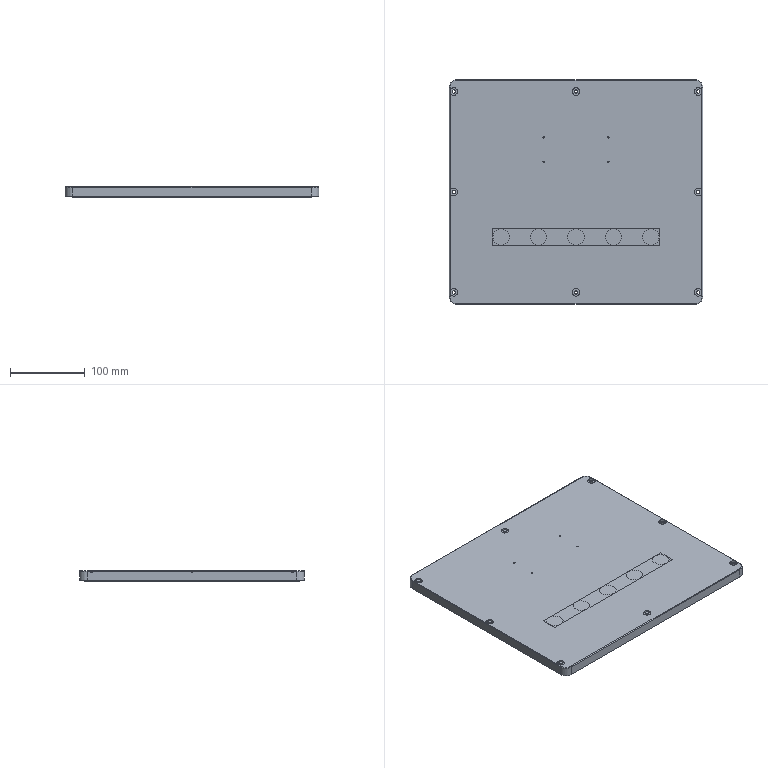NC program | NX | posted with a generic post | part box 338 x 300 x 14.5 mm
Lines 2037 to 2954 of 2954:
(ZLEVEL_PROFILE , TOOL : D10JING)
N4042 T14 M6
N4044 G54
N4046 G17 G0 G90 X160.684 Y-156.916 S9500 M3
N4048 G43 Z30. H14
N4050 Z-11.5
N4052 G94 G1 Z-14.5 F1000.
N4054 X159.866 Y-155.5
N4056 G3 X159. Y-155. R1.
N4058 G1 X-159.
N4060 G2 X-174. Y-140. R15.
N4062 G1 Y140.
N4064 G2 X-159. Y155. R15.
N4066 G1 X159.
N4068 G2 X174. Y140. R15.
N4070 G1 Y-140.
N4072 G2 X159. Y-155. R15.
N4074 G3 X158.134 Y-155.5 R1.
N4076 G1 X157.268 Y-157.
N4078 Z-11.5
N4080 G0 Z30.
(ZLEVEL_PROFILE_COPY , TOOL : D10JING)
N4082 X-52.063 Y-63.427
N4084 Z-2.
N4086 G1 Z-5.
N4088 X-50.866 Y-65.5
N4090 G3 X-50. Y-66. R1.
N4092 X-44. Y-60. R6.
N4094 X-50. Y-66. R-6.
N4096 X-49.134 Y-65.5 R1.
N4098 G1 X-47.937 Y-63.427
N4100 Z-2.
N4102 G0 Z53.
N4104 X-103.427 Y-57.937
N4106 Z-2.
N4108 G1 Z-5.
N4110 X-105.5 Y-59.134
N4112 G3 X-106. Y-60. R1.
N4114 X-100. Y-66. R6.
N4116 X-106. Y-60. R-6.
N4118 X-105.5 Y-60.866 R1.
N4120 G1 X-103.427 Y-62.063
N4122 Z-2.
N4124 G0 Z53.
N4126 X47.937 Y-63.427
N4128 Z-2.
N4130 G1 Z-5.
N4132 X49.134 Y-65.5
N4134 G3 X50. Y-66. R1.
N4136 X56. Y-60. R6.
N4138 X50. Y-66. R-6.
N4140 X50.866 Y-65.5 R1.
N4142 G1 X52.063 Y-63.427
N4144 Z-2.
N4146 G0 Z53.
N4148 X-2.063
N4150 Z-2.
N4152 G1 Z-5.
N4154 X-0.866 Y-65.5
N4156 G3 X0. Y-66. R1.
N4158 X6. Y-60. R6.
N4160 X0. Y-66. R-6.
N4162 X0.866 Y-65.5 R1.
N4164 G1 X2.063 Y-63.427
N4166 Z-2.
N4168 G0 Z53.
N4170 X103.427 Y-62.063
N4172 Z-2.
N4174 G1 Z-5.
N4176 X105.5 Y-60.866
N4178 G3 X106. Y-60. R1.
N4180 X100. Y-54. R6.
N4182 X106. Y-60. R-6.
N4184 X105.5 Y-59.134 R1.
N4186 G1 X103.427 Y-57.937
N4188 Z-2.
N4190 G0 Z30.
N4192 M5
(ZLEVEL_PROFILE_1 , TOOL : D3R0.5)
N4194 T07 M6
N4196 G54
N4198 G17 G0 G90 X-0.52 Y150.79 S9500 M3
N4200 G43 Z30. H7
N4202 Z0.988
N4204 G94 G1 Z-0.012 F1000.
N4206 X-0.26 Y150.34
N4208 G3 X0. Y150.19 R0.3
N4210 G1 X159. F2500.
N4212 G2 X169.19 Y140. R10.19
N4214 G1 Y-140.
N4216 G2 X159. Y-150.19 R10.19
N4218 G1 X-159.
N4220 G2 X-169.19 Y-140. R10.19
N4222 G1 Y140.
N4224 G2 X-159. Y150.19 R10.19
N4226 G1 X0.
N4228 Y150.251 Z-0.021
N4230 Y150.3 Z-0.03
N4232 X-159.
N4234 G3 X-169.3 Y140. R10.3
N4236 G1 Y-140.
N4238 G3 X-159. Y-150.3 R10.3
N4240 G1 X159.
N4242 G3 X169.3 Y-140. R10.3
N4244 G1 Y140.
N4246 G3 X159. Y150.3 R10.3
N4248 G1 X0.
N4250 Y150.356 Z-0.043
N4252 Y150.403 Z-0.055
N4254 X159.
N4256 G2 X169.403 Y140. R10.403
N4258 G1 Y-140.
N4260 G2 X159. Y-150.403 R10.403
N4262 G1 X-159.
N4264 G2 X-169.403 Y-140. R10.403
N4266 G1 Y140.
N4268 G2 X-159. Y150.403 R10.403
N4270 G1 X0.
N4272 Y150.455 Z-0.071
N4274 Y150.502 Z-0.086
N4276 X-159.
N4278 G3 X-169.502 Y140. R10.502
N4280 G1 Y-140.
N4282 G3 X-159. Y-150.502 R10.502
N4284 G1 X159.
N4286 G3 X169.502 Y-140. R10.502
N4288 G1 Y140.
N4290 G3 X159. Y150.502 R10.502
N4292 G1 X0.
N4294 Y150.552 Z-0.105
N4296 Y150.597 Z-0.124
N4298 X159.
N4300 G2 X169.597 Y140. R10.597
N4302 G1 Y-140.
N4304 G2 X159. Y-150.597 R10.597
N4306 G1 X-159.
N4308 G2 X-169.597 Y-140. R10.597
N4310 G1 Y140.
N4312 G2 X-159. Y150.597 R10.597
N4314 G1 X0.
N4316 Y150.645 Z-0.146
N4318 Y150.689 Z-0.167
N4320 X-159.
N4322 G3 X-169.689 Y140. R10.689
N4324 G1 Y-140.
N4326 G3 X-159. Y-150.689 R10.689
N4328 G1 X159.
N4330 G3 X169.689 Y-140. R10.689
N4332 G1 Y140.
N4334 G3 X159. Y150.689 R10.689
N4336 G1 X0.
N4338 Y150.734 Z-0.192
N4340 Y150.777 Z-0.217
N4342 X159.
N4344 G2 X169.777 Y140. R10.777
N4346 G1 Y-140.
N4348 G2 X159. Y-150.777 R10.777
N4350 G1 X-159.
N4352 G2 X-169.777 Y-140. R10.777
N4354 G1 Y140.
N4356 G2 X-159. Y150.777 R10.777
N4358 G1 X0.
N4360 Y150.821 Z-0.244
N4362 Y150.861 Z-0.272
N4364 X-159.
N4366 G3 X-169.861 Y140. R10.861
N4368 G1 Y-140.
N4370 G3 X-159. Y-150.861 R10.861
N4372 G1 X159.
N4374 G3 X169.861 Y-140. R10.861
N4376 G1 Y140.
N4378 G3 X159. Y150.861 R10.861
N4380 G1 X0.
N4382 Y150.903 Z-0.302
N4384 Y150.942 Z-0.333
N4386 X159.
N4388 G2 X169.942 Y140. R10.942
N4390 G1 Y-140.
N4392 G2 X159. Y-150.942 R10.942
N4394 G1 X-159.
N4396 G2 X-169.942 Y-140. R10.942
N4398 G1 Y140.
N4400 G2 X-159. Y150.942 R10.942
N4402 G1 X0.
N4404 Y150.981 Z-0.365
N4406 Y151.018 Z-0.398
N4408 X-159.
N4410 G3 X-170.018 Y140. R11.018
N4412 G1 Y-140.
N4414 G3 X-159. Y-151.018 R11.018
N4416 G1 X159.
N4418 G3 X170.018 Y-140. R11.018
N4420 G1 Y140.
N4422 G3 X159. Y151.018 R11.018
N4424 G1 X0.
N4426 Y151.055 Z-0.434
N4428 Y151.089 Z-0.469
N4430 X159.
N4432 G2 X170.089 Y140. R11.089
N4434 G1 Y-140.
N4436 G2 X159. Y-151.089 R11.089
N4438 G1 X-159.
N4440 G2 X-170.089 Y-140. R11.089
N4442 G1 Y140.
N4444 G2 X-159. Y151.089 R11.089
N4446 G1 X0.
N4448 Y151.124 Z-0.506
N4450 Y151.156 Z-0.544
N4452 X-159.
N4454 G3 X-170.156 Y140. R11.156
N4456 G1 Y-140.
N4458 G3 X-159. Y-151.156 R11.156
N4460 G1 X159.
N4462 G3 X170.156 Y-140. R11.156
N4464 G1 Y140.
N4466 G3 X159. Y151.156 R11.156
N4468 G1 X0.
N4470 Y151.188 Z-0.584
N4472 Y151.217 Z-0.623
N4474 X159.
N4476 G2 X170.217 Y140. R11.217
N4478 G1 Y-140.
N4480 G2 X159. Y-151.217 R11.217
N4482 G1 X-159.
N4484 G2 X-170.217 Y-140. R11.217
N4486 G1 Y140.
N4488 G2 X-159. Y151.217 R11.217
N4490 G1 X0.
N4492 Y151.246 Z-0.665
N4494 Y151.273 Z-0.707
N4496 X-159.
N4498 G3 X-170.273 Y140. R11.273
N4500 G1 Y-140.
N4502 G3 X-159. Y-151.273 R11.273
N4504 G1 X159.
N4506 G3 X170.273 Y-140. R11.273
N4508 G1 Y140.
N4510 G3 X159. Y151.273 R11.273
N4512 G1 X0.
N4514 Y151.299 Z-0.75
N4516 Y151.323 Z-0.793
N4518 X159.
N4520 G2 X170.323 Y140. R11.323
N4522 G1 Y-140.
N4524 G2 X159. Y-151.323 R11.323
N4526 G1 X-159.
N4528 G2 X-170.323 Y-140. R11.323
N4530 G1 Y140.
N4532 G2 X-159. Y151.323 R11.323
N4534 G1 X0.
N4536 Y151.346 Z-0.838
N4538 Y151.367 Z-0.883
N4540 X-159.
N4542 G3 X-170.367 Y140. R11.367
N4544 G1 Y-140.
N4546 G3 X-159. Y-151.367 R11.367
N4548 G1 X159.
N4550 G3 X170.367 Y-140. R11.367
N4552 G1 Y140.
N4554 G3 X159. Y151.367 R11.367
N4556 G1 X0.
N4558 Y151.387 Z-0.93
N4560 Y151.405 Z-0.976
N4562 X159.
N4564 G2 X170.405 Y140. R11.405
N4566 G1 Y-140.
N4568 G2 X159. Y-151.405 R11.405
N4570 G1 X-159.
N4572 G2 X-170.405 Y-140. R11.405
N4574 G1 Y140.
N4576 G2 X-159. Y151.405 R11.405
N4578 G1 X0.
N4580 Y151.422 Z-1.023
N4582 Y151.437 Z-1.071
N4584 X-159.
N4586 G3 X-170.437 Y140. R11.437
N4588 G1 Y-140.
N4590 G3 X-159. Y-151.437 R11.437
N4592 G1 X159.
N4594 G3 X170.437 Y-140. R11.437
N4596 G1 Y140.
N4598 G3 X159. Y151.437 R11.437
N4600 G1 X0.
N4602 Y151.451 Z-1.119
N4604 Y151.463 Z-1.168
N4606 X159.
N4608 G2 X170.463 Y140. R11.463
N4610 G1 Y-140.
N4612 G2 X159. Y-151.463 R11.463
N4614 G1 X-159.
N4616 G2 X-170.463 Y-140. R11.463
N4618 G1 Y140.
N4620 G2 X-159. Y151.463 R11.463
N4622 G1 X0.
N4624 Y151.472 Z-1.209
N4626 Y151.479 Z-1.251
N4628 X-159.
N4630 G3 X-170.479 Y140. R11.479
N4632 G1 Y-140.
N4634 G3 X-159. Y-151.479 R11.479
N4636 G1 X159.
N4638 G3 X170.479 Y-140. R11.479
N4640 G1 Y140.
N4642 G3 X159. Y151.479 R11.479
N4644 G1 X0.
N4646 Y151.486 Z-1.292
N4648 Y151.491 Z-1.334
N4650 X159.
N4652 G2 X170.491 Y140. R11.491
N4654 G1 Y-140.
N4656 G2 X159. Y-151.491 R11.491
N4658 G1 X-159.
N4660 G2 X-170.491 Y-140. R11.491
N4662 G1 Y140.
N4664 G2 X-159. Y151.491 R11.491
N4666 G1 X0.
N4668 Y151.498 Z-1.417
N4670 X-159.
N4672 G3 X-168.723 Y146.136 R11.498
N4674 G1 X-168.807 Y146.001
N4676 G3 X-169.276 Y145.157 R11.498
N4678 G1 X-169.297 Y145.116
N4680 G3 X-169.508 Y144.667 R11.498
N4682 G1 X-169.542 Y144.59
N4684 G3 X-169.712 Y144.178 R11.498
N4686 G1 X-169.786 Y143.981
N4688 G3 X-169.89 Y143.688 R11.498
N4690 G1 X-170.031 Y143.242
N4692 G3 X-170.231 Y142.464 R11.498
N4694 G1 X-170.276 Y142.247
N4696 G3 X-170.401 Y141.485 R11.498
N4698 G1 X-170.417 Y141.363
N4700 G3 X-170.495 Y140.261 R11.498
N4702 G1 X-170.497 Y140.139
N4704 X-170.498 Y140.
N4706 Y-140.
N4708 X-170.497 Y-140.126
N4710 X-170.491 Y-140.383
N4712 G3 X-170.421 Y-141.323 R11.498
N4714 G1 X-170.401 Y-141.485
N4716 G3 X-170.276 Y-142.247 R11.498
N4718 G1 X-170.203 Y-142.587
N4720 G3 X-170.031 Y-143.242 R11.498
N4722 G1 X-169.848 Y-143.811
N4724 X-169.786 Y-143.981
N4726 X-169.712 Y-144.178
N4728 G3 X-169.542 Y-144.59 R11.498
N4730 G1 X-169.452 Y-144.79
N4732 G3 X-169.297 Y-145.116 R11.498
N4734 G1 X-169.214 Y-145.28
N4736 G3 X-168.807 Y-146.001 R11.498
N4738 G1 X-168.645 Y-146.259
N4740 G3 X-167.454 Y-147.792 R11.498
N4742 G1 X-167.338 Y-147.916
N4744 G3 X-166.979 Y-148.278 R11.498
N4746 G1 X-166.849 Y-148.402
N4748 G3 X-165.252 Y-149.65 R11.498
N4750 G1 X-165.001 Y-149.808
N4752 G3 X-164.289 Y-150.209 R11.498
N4754 G1 X-164.115 Y-150.297
N4756 G3 X-163.666 Y-150.508 R11.498
N4758 G1 X-163.59 Y-150.542
N4760 G3 X-163.268 Y-150.676 R11.498
N4762 G1 X-162.98 Y-150.787
N4764 X-162.812 Y-150.847
N4766 X-162.241 Y-151.032
N4768 G3 X-160.483 Y-151.402 R11.498
N4770 G1 X-160.116 Y-151.443
N4772 G3 X-159.376 Y-151.492 R11.498
N4774 G1 X159.014 Y-151.496
N4776 X159.381 Y-151.491
N4778 G3 X160.045 Y-151.45 R11.498
N4780 G1 X160.483 Y-151.402
N4782 G3 X161.245 Y-151.276 R11.498
N4784 G1 X161.83 Y-151.144
N4786 G3 X162.241 Y-151.032 R11.498
N4788 G1 X162.809 Y-150.848
N4790 X162.98 Y-150.787
N4792 X163.176 Y-150.712
N4794 G3 X163.59 Y-150.542 R11.498
N4796 G1 X163.666 Y-150.508
N4798 G3 X164.115 Y-150.297 R11.498
N4800 G1 X164.278 Y-150.214
N4802 G3 X165.001 Y-149.808 R11.498
N4804 G1 X165.258 Y-149.646
N4806 G3 X166.789 Y-148.458 R11.498
N4808 G1 X166.849 Y-148.402
N4810 G3 X167.279 Y-147.978 R11.498
N4812 G1 X167.338 Y-147.916
N4814 G3 X170.498 Y-140. R11.498
N4816 G1 Y140.
N4818 G3 X159. Y151.498 R11.498
N4820 G1 X0.
N4822 Y151.499 Z-1.5
N4824 X159.014
N4826 G2 X170.5 Y140.016 R11.501
N4828 G1 Y-140.016
N4830 G2 X167.338 Y-147.916 R11.492
N4832 G1 X167.279 Y-147.978
N4834 G2 X165.258 Y-149.646 R10.784
N4836 X163.872 Y-150.411 R10.382
N4838 X159.452 Y-151.49 R11.348
N4840 G1 X159.014 Y-151.498
N4842 X-159.014
N4844 X-159.376 Y-151.492
N4846 X-159.993 Y-151.456
N4848 X-160.317 Y-151.424
N4850 G2 X-162.616 Y-150.912 R11.252
N4852 G1 X-163.217 Y-150.71
N4854 G2 X-164.876 Y-149.895 R17.007
N4856 X-166.979 Y-148.278 R12.287
N4858 X-168.645 Y-146.259 R10.898
N4860 X-169.214 Y-145.28 R10.966
N4862 X-169.848 Y-143.811 R10.939
N4864 X-170.203 Y-142.587 R11.162
N4866 X-170.401 Y-141.485 R10.8
N4868 X-170.491 Y-140.383 R10.626
N4870 G1 X-170.497 Y-140.126
N4872 X-170.499 Y139.772
N4874 X-170.495 Y140.261
N4876 G2 X-170.401 Y141.485 R10.805
N4878 X-169.941 Y143.58 R13.259
N4880 X-169.382 Y144.948 R17.018
N4882 X-168.723 Y146.136 R10.907
N4884 X-167.401 Y147.85 R11.101
N4886 G1 X-167.338 Y147.918
N4888 X-166.916 Y148.339
N4890 G2 X-159. Y151.5 R11.492
N4892 G1 X0. Y151.499
N4894 G3 X0.26 Y151.649 R0.3
N4896 G1 X0.52 Y152.099
N4898 Z-0.5
N4900 G0 Z30.
N4902 M5
(HOLE_MILLING_1 , TOOL : D6)
N4904 T16 M6
N4906 G54
N4908 G17 G0 G90 X-163. Y134. S9500 M3
N4910 G43 Z30. H16
N4912 Z0.5
N4914 G94 G3 X-162. Y133. R1. F1400.
N4916 X-161. Y134. R1.
N4918 X-161. Y134. Z0. I-2. J0.
N4920 X-161. Y134. Z-0.5 I-2. J0.
N4922 X-161. Y134. Z-1. I-2. J0.
N4924 X-161. Y134. Z-1.5 I-2. J0.
N4926 X-161. Y134. Z-2. I-2. J0.
N4928 X-163. Y136. R2.
N4930 X-161. Y134. R-2.
N4932 X-162. Y135. R1.
N4934 X-163. Y134. R1.
N4936 G0 Z30.
N4938 Y0.
N4940 Z0.5
N4942 G3 X-162. Y-1. R1.
N4944 X-161. Y0. R1.
N4946 X-161. Y0. Z0. I-2. J0.
N4948 X-161. Y0. Z-0.5 I-2. J0.
N4950 X-161. Y0. Z-1. I-2. J0.
N4952 X-161. Y0. Z-1.5 I-2. J0.
N4954 X-161. Y0. Z-2. I-2. J0.
N4956 X-163. Y2. R2.
N4958 X-161. Y0. R-2.
N4960 X-162. Y1. R1.
N4962 X-163. Y0. R1.
N4964 G0 Z30.
N4966 Y-134.
N4968 Z0.5
N4970 G3 X-162. Y-135. R1.
N4972 X-161. Y-134. R1.
N4974 X-161. Y-134. Z0. I-2. J0.
N4976 X-161. Y-134. Z-0.5 I-2. J0.
N4978 X-161. Y-134. Z-1. I-2. J0.
N4980 X-161. Y-134. Z-1.5 I-2. J0.
N4982 X-161. Y-134. Z-2. I-2. J0.
N4984 X-163. Y-132. R2.
N4986 X-161. Y-134. R-2.
N4988 X-162. Y-133. R1.
N4990 X-163. Y-134. R1.
N4992 G0 Z30.
N4994 X0.
N4996 Z0.5
N4998 G3 X1. Y-135. R1.
N5000 X2. Y-134. R1.
N5002 X2. Y-134. Z0. I-2. J0.
N5004 X2. Y-134. Z-0.5 I-2. J0.
N5006 X2. Y-134. Z-1. I-2. J0.
N5008 X2. Y-134. Z-1.5 I-2. J0.
N5010 X2. Y-134. Z-2. I-2. J0.
N5012 X0. Y-132. R2.
N5014 X2. Y-134. R-2.
N5016 X1. Y-133. R1.
N5018 X0. Y-134. R1.
N5020 G0 Z30.
N5022 X163.
N5024 Z0.5
N5026 G3 X164. Y-135. R1.
N5028 X165. Y-134. R1.
N5030 X165. Y-134. Z0. I-2. J0.
N5032 X165. Y-134. Z-0.5 I-2. J0.
N5034 X165. Y-134. Z-1. I-2. J0.
N5036 X165. Y-134. Z-1.5 I-2. J0.
N5038 X165. Y-134. Z-2. I-2. J0.
N5040 X163. Y-132. R2.
N5042 X165. Y-134. R-2.
N5044 X164. Y-133. R1.
N5046 X163. Y-134. R1.
N5048 G0 Z30.
N5050 Y0.
N5052 Z0.5
N5054 G3 X164. Y-1. R1.
N5056 X165. Y0. R1.
N5058 X165. Y0. Z0. I-2. J0.
N5060 X165. Y0. Z-0.5 I-2. J0.
N5062 X165. Y0. Z-1. I-2. J0.
N5064 X165. Y0. Z-1.5 I-2. J0.
N5066 X165. Y0. Z-2. I-2. J0.
N5068 X163. Y2. R2.
N5070 X165. Y0. R-2.
N5072 X164. Y1. R1.
N5074 X163. Y0. R1.
N5076 G0 Z30.
N5078 Y134.
N5080 Z0.5
N5082 G3 X164. Y133. R1.
N5084 X165. Y134. R1.
N5086 X165. Y134. Z0. I-2. J0.
N5088 X165. Y134. Z-0.5 I-2. J0.
N5090 X165. Y134. Z-1. I-2. J0.
N5092 X165. Y134. Z-1.5 I-2. J0.
N5094 X165. Y134. Z-2. I-2. J0.
N5096 X163. Y136. R2.
N5098 X165. Y134. R-2.
N5100 X164. Y135. R1.
N5102 X163. Y134. R1.
N5104 G0 Z30.
N5106 X0.
N5108 Z0.5
N5110 G3 X1. Y133. R1.
N5112 X2. Y134. R1.
N5114 X2. Y134. Z0. I-2. J0.
N5116 X2. Y134. Z-0.5 I-2. J0.
N5118 X2. Y134. Z-1. I-2. J0.
N5120 X2. Y134. Z-1.5 I-2. J0.
N5122 X2. Y134. Z-2. I-2. J0.
N5124 X0. Y136. R2.
N5126 X2. Y134. R-2.
N5128 X1. Y135. R1.
N5130 X0. Y134. R1.
N5132 G0 Z30.
N5134 M5
(PLANAR_MILL_COPY_COPY , TOOL : D6A45)
N5136 T01 M6
N5138 G54
N5140 G17 G0 G90 X-3.351 Y135.01 S9500 M3
N5142 G43 Z30. H1
N5144 Z0.
N5146 G94 G1 Z-1. F1250.
N5148 X-3.6 Y134.866
N5150 G3 X-4.1 Y134. R1.
N5152 X0. Y129.9 R4.1
N5154 X-4.1 Y134. R-4.1
N5156 X-3.6 Y133.134 R1.
N5158 G1 X-3.351 Y132.99
N5160 Z0.
N5162 G0 Z30.
N5164 X43.125 Y73.008
N5166 Z0.
N5168 G1 Y73.051 Z-0.011
N5170 X43.068 Y73.117 Z-0.035
N5172 X42.982 Y73.134 Z-0.058
N5174 X42.893 Y73.083 Z-0.086
N5176 X42.875 Y73.051 Z-0.095
N5178 Y72.949 Z-0.123
N5180 X42.893 Y72.917 Z-0.133
N5182 X42.982 Y72.866 Z-0.16
N5184 X43.068 Y72.883 Z-0.183
N5186 X43.125 Y72.949 Z-0.207
N5188 Y73.051 Z-0.234
N5190 X43.068 Y73.117 Z-0.258
N5192 X42.982 Y73.134 Z-0.281
N5194 X42.893 Y73.083 Z-0.308
N5196 X42.875 Y73.051 Z-0.318
N5198 Y72.949 Z-0.346
N5200 X42.893 Y72.917 Z-0.355
N5202 X42.982 Y72.866 Z-0.383
N5204 X43.068 Y72.883 Z-0.406
N5206 X43.125 Y72.949 Z-0.43
N5208 Y73.051 Z-0.457
N5210 X43.068 Y73.117 Z-0.48
N5212 X42.982 Y73.134 Z-0.504
N5214 X42.893 Y73.083 Z-0.531
N5216 X42.875 Y73.051 Z-0.541
N5218 Y72.949 Z-0.568
N5220 X42.893 Y72.917 Z-0.578
N5222 X42.982 Y72.866 Z-0.605
N5224 X43.068 Y72.883 Z-0.629
N5226 X43.125 Y72.949 Z-0.652
N5228 Y73.051 Z-0.68
N5230 X43.068 Y73.117 Z-0.703
N5232 X42.982 Y73.134 Z-0.726
N5234 X42.893 Y73.083 Z-0.754
N5236 X42.875 Y73.051 Z-0.764
N5238 Y72.949 Z-0.791
N5240 X42.893 Y72.917 Z-0.801
N5242 X42.982 Y72.866 Z-0.828
N5244 X43.068 Y72.883 Z-0.852
N5246 X43.125 Y72.949 Z-0.875
N5248 Y73.051 Z-0.902
N5250 X43.068 Y73.117 Z-0.926
N5252 X42.982 Y73.134 Z-0.949
N5254 X42.893 Y73.083 Z-0.977
N5256 X42.875 Y73.051 Z-0.986
N5258 Y73. Z-1.
N5260 G3 X43. Y72.875 R0.125
N5262 X42.875 Y73. R-0.125
N5264 G1 Z0.
N5266 G0 Z30.
N5268 X43.125 Y40.008
N5270 Z0.
N5272 G1 Y40.051 Z-0.011
N5274 X43.068 Y40.117 Z-0.035
N5276 X42.982 Y40.134 Z-0.058
N5278 X42.893 Y40.083 Z-0.086
N5280 X42.875 Y40.051 Z-0.095
N5282 Y39.949 Z-0.123
N5284 X42.893 Y39.917 Z-0.133
N5286 X42.982 Y39.866 Z-0.16
N5288 X43.068 Y39.883 Z-0.183
N5290 X43.125 Y39.949 Z-0.207
N5292 Y40.051 Z-0.234
N5294 X43.068 Y40.117 Z-0.258
N5296 X42.982 Y40.134 Z-0.281
N5298 X42.893 Y40.083 Z-0.308
N5300 X42.875 Y40.051 Z-0.318
N5302 Y39.949 Z-0.346
N5304 X42.893 Y39.917 Z-0.355
N5306 X42.982 Y39.866 Z-0.383
N5308 X43.068 Y39.883 Z-0.406
N5310 X43.125 Y39.949 Z-0.43
N5312 Y40.051 Z-0.457
N5314 X43.068 Y40.117 Z-0.48
N5316 X42.982 Y40.134 Z-0.504
N5318 X42.893 Y40.083 Z-0.531
N5320 X42.875 Y40.051 Z-0.541
N5322 Y39.949 Z-0.568
N5324 X42.893 Y39.917 Z-0.578
N5326 X42.982 Y39.866 Z-0.605
N5328 X43.068 Y39.883 Z-0.629
N5330 X43.125 Y39.949 Z-0.652
N5332 Y40.051 Z-0.68
N5334 X43.068 Y40.117 Z-0.703
N5336 X42.982 Y40.134 Z-0.726
N5338 X42.893 Y40.083 Z-0.754
N5340 X42.875 Y40.051 Z-0.764
N5342 Y39.949 Z-0.791
N5344 X42.893 Y39.917 Z-0.801
N5346 X42.982 Y39.866 Z-0.828
N5348 X43.068 Y39.883 Z-0.852
N5350 X43.125 Y39.949 Z-0.875
N5352 Y40.051 Z-0.902
N5354 X43.068 Y40.117 Z-0.926
N5356 X42.982 Y40.134 Z-0.949
N5358 X42.893 Y40.083 Z-0.977
N5360 X42.875 Y40.051 Z-0.986
N5362 Y40. Z-1.
N5364 G3 X43. Y39.875 R0.125
N5366 X42.875 Y40. R-0.125
N5368 G1 Z0.
N5370 G0 Z30.
N5372 X-42.875 Y40.008
N5374 Z0.
N5376 G1 Y40.051 Z-0.011
N5378 X-42.933 Y40.117 Z-0.035
N5380 X-43.018 Y40.134 Z-0.058
N5382 X-43.107 Y40.083 Z-0.086
N5384 X-43.125 Y40.051 Z-0.095
N5386 Y39.949 Z-0.123
N5388 X-43.107 Y39.917 Z-0.133
N5390 X-43.018 Y39.866 Z-0.16
N5392 X-42.933 Y39.883 Z-0.183
N5394 X-42.875 Y39.949 Z-0.207
N5396 Y40.051 Z-0.234
N5398 X-42.933 Y40.117 Z-0.258
N5400 X-43.018 Y40.134 Z-0.281
N5402 X-43.107 Y40.083 Z-0.308
N5404 X-43.125 Y40.051 Z-0.318
N5406 Y39.949 Z-0.346
N5408 X-43.107 Y39.917 Z-0.355
N5410 X-43.018 Y39.866 Z-0.383
N5412 X-42.933 Y39.883 Z-0.406
N5414 X-42.875 Y39.949 Z-0.43
N5416 Y40.051 Z-0.457
N5418 X-42.933 Y40.117 Z-0.48
N5420 X-43.018 Y40.134 Z-0.504
N5422 X-43.107 Y40.083 Z-0.531
N5424 X-43.125 Y40.051 Z-0.541
N5426 Y39.949 Z-0.568
N5428 X-43.107 Y39.917 Z-0.578
N5430 X-43.018 Y39.866 Z-0.605
N5432 X-42.933 Y39.883 Z-0.629
N5434 X-42.875 Y39.949 Z-0.652
N5436 Y40.051 Z-0.68
N5438 X-42.933 Y40.117 Z-0.703
N5440 X-43.018 Y40.134 Z-0.726
N5442 X-43.107 Y40.083 Z-0.754
N5444 X-43.125 Y40.051 Z-0.764
N5446 Y39.949 Z-0.791
N5448 X-43.107 Y39.917 Z-0.801
N5450 X-43.018 Y39.866 Z-0.828
N5452 X-42.933 Y39.883 Z-0.852
N5454 X-42.875 Y39.949 Z-0.875
N5456 Y40.051 Z-0.902
N5458 X-42.933 Y40.117 Z-0.926
N5460 X-43.018 Y40.134 Z-0.949
N5462 X-43.107 Y40.083 Z-0.977
N5464 X-43.125 Y40.051 Z-0.986
N5466 Y40. Z-1.
N5468 G3 X-43. Y39.875 R0.125
N5470 X-43.125 Y40. R-0.125
N5472 G1 Z0.
N5474 G0 Z30.
N5476 X-42.875 Y73.008
N5478 Z0.
N5480 G1 Y73.051 Z-0.011
N5482 X-42.933 Y73.117 Z-0.035
N5484 X-43.018 Y73.134 Z-0.058
N5486 X-43.107 Y73.083 Z-0.086
N5488 X-43.125 Y73.051 Z-0.095
N5490 Y72.949 Z-0.123
N5492 X-43.107 Y72.917 Z-0.133
N5494 X-43.018 Y72.866 Z-0.16
N5496 X-42.933 Y72.883 Z-0.183
N5498 X-42.875 Y72.949 Z-0.207
N5500 Y73.051 Z-0.234
N5502 X-42.933 Y73.117 Z-0.258
N5504 X-43.018 Y73.134 Z-0.281
N5506 X-43.107 Y73.083 Z-0.308
N5508 X-43.125 Y73.051 Z-0.318
N5510 Y72.949 Z-0.346
N5512 X-43.107 Y72.917 Z-0.355
N5514 X-43.018 Y72.866 Z-0.383
N5516 X-42.933 Y72.883 Z-0.406
N5518 X-42.875 Y72.949 Z-0.43
N5520 Y73.051 Z-0.457
N5522 X-42.933 Y73.117 Z-0.48
N5524 X-43.018 Y73.134 Z-0.504
N5526 X-43.107 Y73.083 Z-0.531
N5528 X-43.125 Y73.051 Z-0.541
N5530 Y72.949 Z-0.568
N5532 X-43.107 Y72.917 Z-0.578
N5534 X-43.018 Y72.866 Z-0.605
N5536 X-42.933 Y72.883 Z-0.629
N5538 X-42.875 Y72.949 Z-0.652
N5540 Y73.051 Z-0.68
N5542 X-42.933 Y73.117 Z-0.703
N5544 X-43.018 Y73.134 Z-0.726
N5546 X-43.107 Y73.083 Z-0.754
N5548 X-43.125 Y73.051 Z-0.764
N5550 Y72.949 Z-0.791
N5552 X-43.107 Y72.917 Z-0.801
N5554 X-43.018 Y72.866 Z-0.828
N5556 X-42.933 Y72.883 Z-0.852
N5558 X-42.875 Y72.949 Z-0.875
N5560 Y73.051 Z-0.902
N5562 X-42.933 Y73.117 Z-0.926
N5564 X-43.018 Y73.134 Z-0.949
N5566 X-43.107 Y73.083 Z-0.977
N5568 X-43.125 Y73.051 Z-0.986
N5570 Y73. Z-1.
N5572 G3 X-43. Y72.875 R0.125
N5574 X-43.125 Y73. R-0.125
N5576 G1 Z0.
N5578 G0 Z30.
N5580 X-166.351 Y135.01
N5582 Z0.
N5584 G1 Z-1.
N5586 X-166.6 Y134.866
N5588 G3 X-167.1 Y134. R1.
N5590 X-163. Y129.9 R4.1
N5592 X-167.1 Y134. R-4.1
N5594 X-166.6 Y133.134 R1.
N5596 G1 X-166.351 Y132.99
N5598 Z0.
N5600 G0 Z30.
N5602 Y1.01
N5604 Z0.
N5606 G1 Z-1.
N5608 X-166.6 Y0.866
N5610 G3 X-167.1 Y0. R1.
N5612 X-163. Y-4.1 R4.1
N5614 X-167.1 Y0. R-4.1
N5616 X-166.6 Y-0.866 R1.
N5618 G1 X-166.351 Y-1.01
N5620 Z0.
N5622 G0 Z30.
N5624 Y-132.99
N5626 Z0.
N5628 G1 Z-1.
N5630 X-166.6 Y-133.134
N5632 G3 X-167.1 Y-134. R1.
N5634 X-163. Y-138.1 R4.1
N5636 X-167.1 Y-134. R-4.1
N5638 X-166.6 Y-134.866 R1.
N5640 G1 X-166.351 Y-135.01
N5642 Z0.
N5644 G0 Z30.
N5646 X-90.548 Y-60.951
N5648 Z0.
N5650 G1 Z-1.
N5652 X-90.4 Y-60.866
N5654 G3 X-89.9 Y-60. R1.
N5656 X-100. Y-49.9 R10.1
N5658 X-89.9 Y-60. R-10.1
N5660 X-90.4 Y-59.134 R1.
N5662 G1 X-90.548 Y-59.049
N5664 Z0.
N5666 G0 Z30.
N5668 X-40.548 Y-60.951
N5670 Z0.
N5672 G1 Z-1.
N5674 X-40.4 Y-60.866
N5676 G3 X-39.9 Y-60. R1.
N5678 X-50. Y-49.9 R10.1
N5680 X-39.9 Y-60. R-10.1
N5682 X-40.4 Y-59.134 R1.
N5684 G1 X-40.548 Y-59.049
N5686 Z0.
N5688 G0 Z30.
N5690 X-3.351 Y-132.99
N5692 Z0.
N5694 G1 Z-1.
N5696 X-3.6 Y-133.134
N5698 G3 X-4.1 Y-134. R1.
N5700 X0. Y-138.1 R4.1
N5702 X-4.1 Y-134. R-4.1
N5704 X-3.6 Y-134.866 R1.
N5706 G1 X-3.351 Y-135.01
N5708 Z0.
N5710 G0 Z30.
N5712 X9.452 Y-60.951
N5714 Z0.
N5716 G1 Z-1.
N5718 X9.6 Y-60.866
N5720 G3 X10.1 Y-60. R1.
N5722 X0. Y-49.9 R10.1
N5724 X10.1 Y-60. R-10.1
N5726 X9.6 Y-59.134 R1.
N5728 G1 X9.452 Y-59.049
N5730 Z0.
N5732 G0 Z30.
N5734 X59.452 Y-60.951
N5736 Z0.
N5738 G1 Z-1.
N5740 X59.6 Y-60.866
N5742 G3 X60.1 Y-60. R1.
N5744 X50. Y-49.9 R10.1
N5746 X60.1 Y-60. R-10.1
N5748 X59.6 Y-59.134 R1.
N5750 G1 X59.452 Y-59.049
N5752 Z0.
N5754 G0 Z30.
N5756 X109.452 Y-60.951
N5758 Z0.
N5760 G1 Z-1.
N5762 X109.6 Y-60.866
N5764 G3 X110.1 Y-60. R1.
N5766 X100. Y-49.9 R10.1
N5768 X110.1 Y-60. R-10.1
N5770 X109.6 Y-59.134 R1.
N5772 G1 X109.452 Y-59.049
N5774 Z0.
N5776 G0 Z30.
N5778 X159.649 Y-132.99
N5780 Z0.
N5782 G1 Z-1.
N5784 X159.4 Y-133.134
N5786 G3 X158.9 Y-134. R1.
N5788 X163. Y-138.1 R4.1
N5790 X158.9 Y-134. R-4.1
N5792 X159.4 Y-134.866 R1.
N5794 G1 X159.649 Y-135.01
N5796 Z0.
N5798 G0 Z30.
N5800 Y1.01
N5802 Z0.
N5804 G1 Z-1.
N5806 X159.4 Y0.866
N5808 G3 X158.9 Y0. R1.
N5810 X163. Y-4.1 R4.1
N5812 X158.9 Y0. R-4.1
N5814 X159.4 Y-0.866 R1.
N5816 G1 X159.649 Y-1.01
N5818 Z0.
N5820 G0 Z30.
N5822 Y135.01
N5824 Z0.
N5826 G1 Z-1.
N5828 X159.4 Y134.866
N5830 G3 X158.9 Y134. R1.
N5832 X163. Y129.9 R4.1
N5834 X158.9 Y134. R-4.1
N5836 X159.4 Y133.134 R1.
N5838 G1 X159.649 Y132.99
N5840 Z0.
N5842 G0 Z30.
N5844 M5
N5846 M2